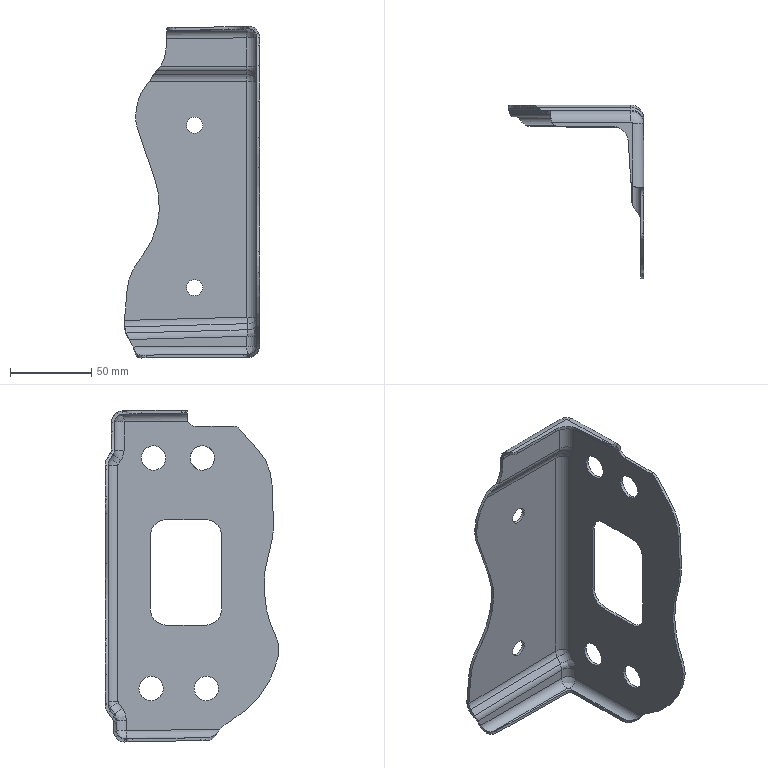Part | 1 solid | 127 faces | box 83.346 x 106.928 x 204.549 mm | volume 53980 mm3 | cylinder 56 | spline 43 | plane 24 | torus 2 | other 2 | commonest cylinder face diameters 10 x11 15 x8 12 x5 15.6 x5 13.6 x4 20 x4